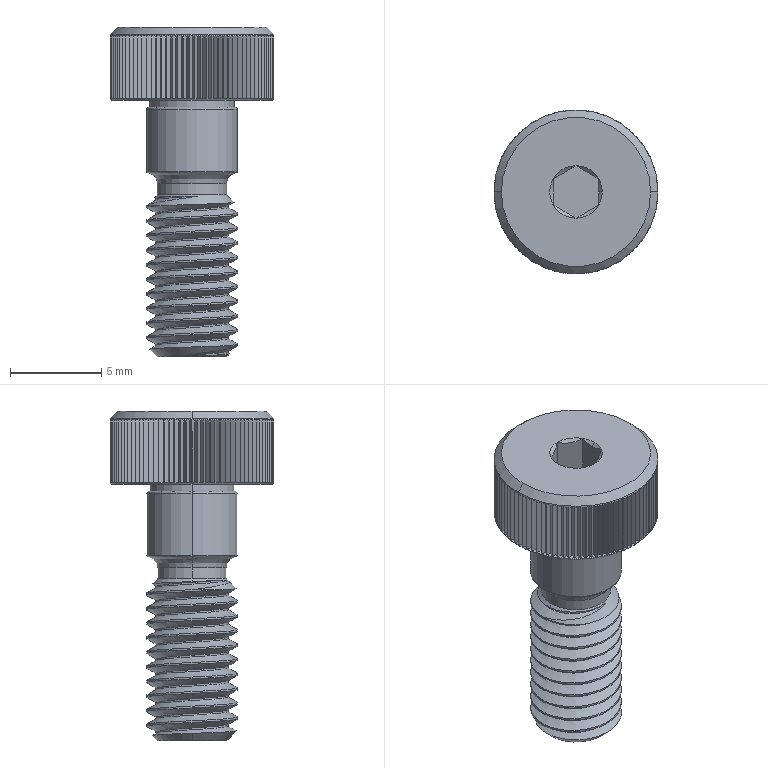Part | NX | features solid 2 | 1 solid | 426 faces | box 9.002 x 9 x 18.1 mm | volume 459.664 mm3 | plane 371 | cylinder 31 | cone 13 | torus 8 | spline 3 | commonest cylinder face diameters 5 x23 9 x4 3.8 x2 4.65 x2